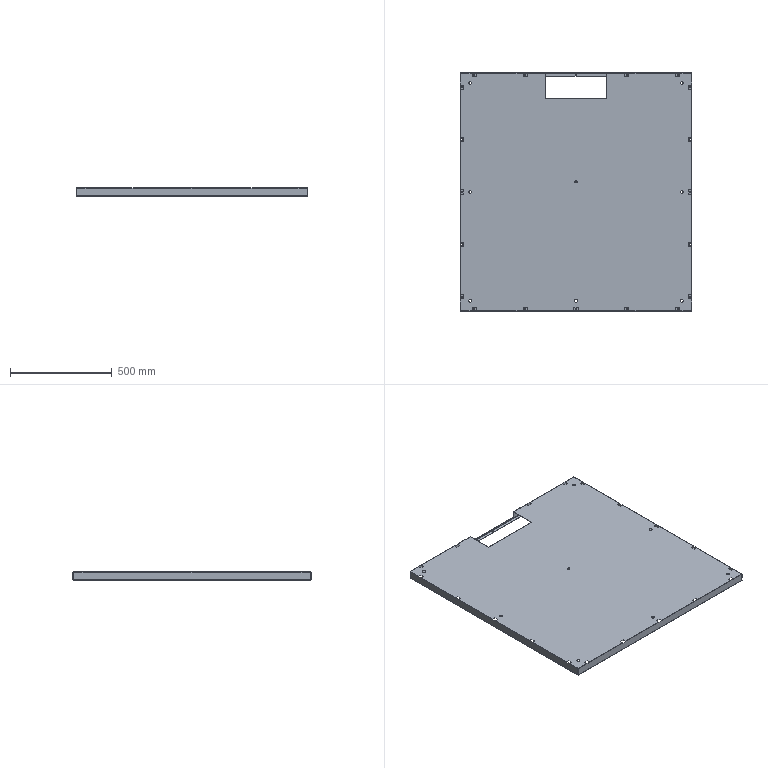Part | 1 solid | 376 faces | box 1139 x 1169 x 40 mm | volume 1525092 mm3 | plane 238 | cylinder 122 | spline 16 | commonest cylinder face diameters 7 x50 0.4 x28 2.4 x28 14 x14 11 x2